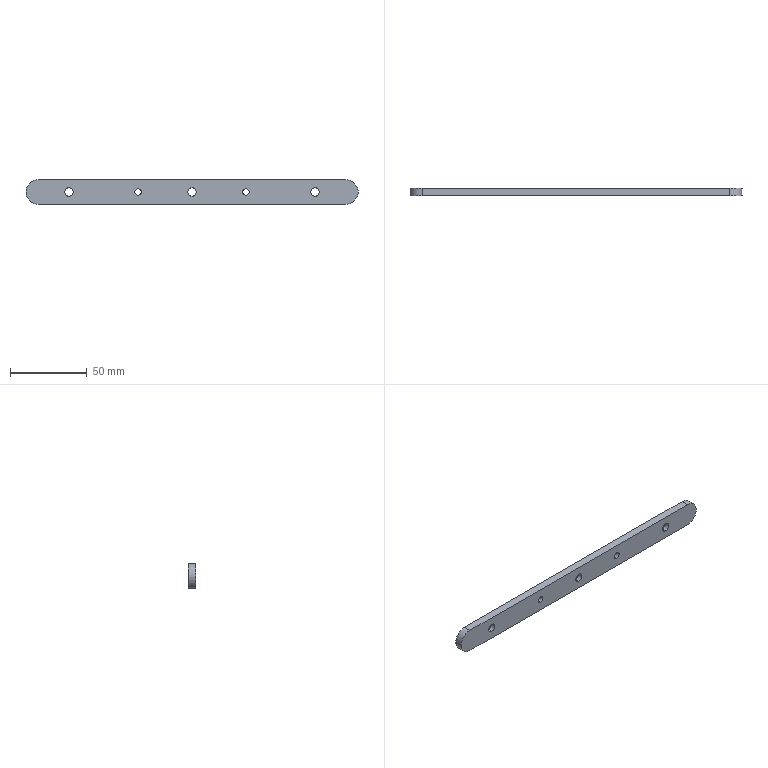Part | STEP file | PN_0027 KEY_Default | 1 solid | 25 faces | box 216 x 5 x 16 mm | volume 16228 mm3 | cylinder 18 | plane 7 | commonest cylinder face diameters 5.5 x6 9.5 x6 4.2 x4 16 x2